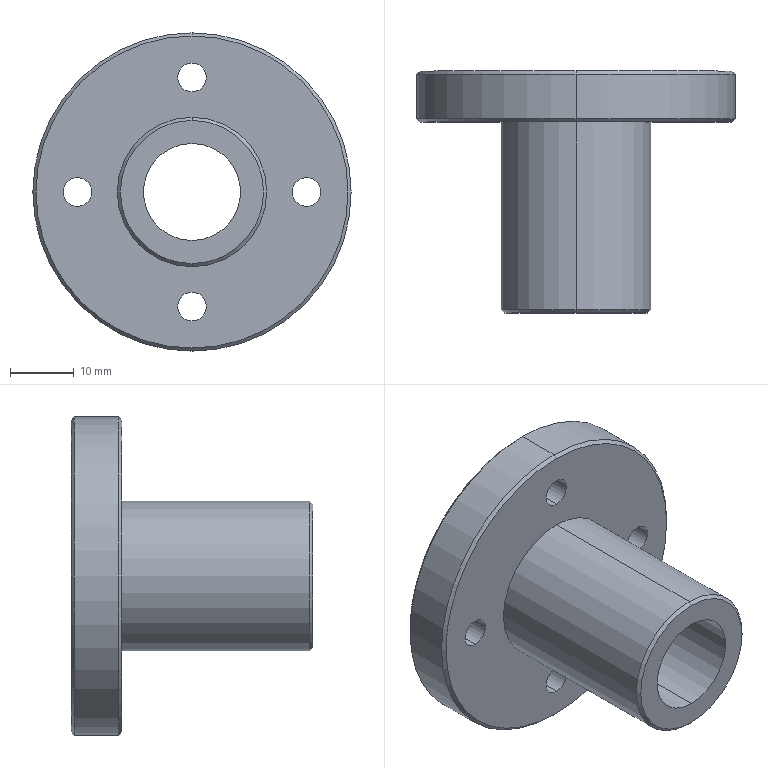Part | SolidWorks | features 3DProfileFeature 3, HoleWzd 3, Chamfer 1, Revolution 1 | 1 solid | 35 faces | box 50 x 38 x 50 mm | volume 20590 mm3 | cylinder 22 | plane 7 | cone 6 | commonest cylinder face diameters 4.5 x8 8 x8 15.25 x2 23.5 x2 50 x2
STEP:
#1=CARTESIAN_POINT('',(0.,38.,24.5));
#2=VERTEX_POINT('',#1);
#3=CARTESIAN_POINT('',(0.,38.,-24.5));
#4=VERTEX_POINT('',#3);
#5=CARTESIAN_POINT('',(0.,38.,0.));
#6=DIRECTION('',(0.,1.,0.));
#7=DIRECTION('',(0.,0.,-1.));
#8=AXIS2_PLACEMENT_3D('',#5,#6,#7);
#9=CIRCLE('',#8,24.5);
#10=EDGE_CURVE('',#2,#4,#9,.T.);
#11=ORIENTED_EDGE('',*,*,#10,.F.);
#12=CARTESIAN_POINT('',(0.,37.5,25.));
#13=VERTEX_POINT('',#12);
#14=CARTESIAN_POINT('',(0.,37.5,25.));
#15=DIRECTION('',(0.,-0.7071,0.7071));
#16=VECTOR('',#15,1000.);
#17=LINE('',#14,#16);
#18=EDGE_CURVE('',#2,#13,#17,.T.);
#19=ORIENTED_EDGE('',*,*,#18,.T.);
#20=CARTESIAN_POINT('',(0.,37.5,-25.));
#21=VERTEX_POINT('',#20);
#22=CARTESIAN_POINT('',(0.,37.5,0.));
#23=DIRECTION('',(0.,-1.,0.));
#24=DIRECTION('',(0.,0.,-1.));
#25=AXIS2_PLACEMENT_3D('',#22,#23,#24);
#26=CIRCLE('',#25,25.);
#27=EDGE_CURVE('',#21,#13,#26,.T.);
#28=ORIENTED_EDGE('',*,*,#27,.F.);
#29=CARTESIAN_POINT('',(0.,37.5,-25.));
#30=DIRECTION('',(0.,-0.7071,-0.7071));
#31=VECTOR('',#30,1000.);
#32=LINE('',#29,#31);
#33=EDGE_CURVE('',#4,#21,#32,.T.);
#34=ORIENTED_EDGE('',*,*,#33,.F.);
#35=EDGE_LOOP('',(#11,#19,#28,#34));
#36=FACE_OUTER_BOUND('',#35,.T.);
#37=CARTESIAN_POINT('',(0.,37.5,0.));
#38=DIRECTION('',(0.,-1.,0.));
#39=DIRECTION('',(0.,0.,-1.));
#40=AXIS2_PLACEMENT_3D('',#37,#38,#39);
#41=CONICAL_SURFACE('',#40,25.,0.7854);
#42=ADVANCED_FACE('',(#36),#41,.T.);
#43=CARTESIAN_POINT('',(0.,30.,-24.5));
#44=VERTEX_POINT('',#43);
#45=CARTESIAN_POINT('',(0.,30.,24.5));
#46=VERTEX_POINT('',#45);
#47=CARTESIAN_POINT('',(0.,30.,0.));
#48=DIRECTION('',(0.,-1.,0.));
#49=DIRECTION('',(0.,0.,1.));
#50=AXIS2_PLACEMENT_3D('',#47,#48,#49);
#51=CIRCLE('',#50,24.5);
#52=EDGE_CURVE('',#44,#46,#51,.T.);
#53=ORIENTED_EDGE('',*,*,#52,.F.);
#54=CARTESIAN_POINT('',(0.,30.5,-25.));
#55=VERTEX_POINT('',#54);
#56=CARTESIAN_POINT('',(0.,30.,-24.5));
#57=DIRECTION('',(0.,0.7071,-0.7071));
#58=VECTOR('',#57,1000.);
#59=LINE('',#56,#58);
#60=EDGE_CURVE('',#44,#55,#59,.T.);
#61=ORIENTED_EDGE('',*,*,#60,.T.);
#62=CARTESIAN_POINT('',(0.,30.5,25.));
#63=VERTEX_POINT('',#62);
#64=CARTESIAN_POINT('',(0.,30.5,0.));
#65=DIRECTION('',(0.,1.,0.));
#66=DIRECTION('',(0.,0.,1.));
#67=AXIS2_PLACEMENT_3D('',#64,#65,#66);
#68=CIRCLE('',#67,25.);
#69=EDGE_CURVE('',#63,#55,#68,.T.);
#70=ORIENTED_EDGE('',*,*,#69,.F.);
#71=CARTESIAN_POINT('',(0.,30.,24.5));
#72=DIRECTION('',(0.,0.7071,0.7071));
#73=VECTOR('',#72,1000.);
#74=LINE('',#71,#73);
#75=EDGE_CURVE('',#46,#63,#74,.T.);
#76=ORIENTED_EDGE('',*,*,#75,.F.);
#77=EDGE_LOOP('',(#53,#61,#70,#76));
#78=FACE_OUTER_BOUND('',#77,.T.);
#79=CARTESIAN_POINT('',(0.,30.,0.));
#80=DIRECTION('',(0.,1.,0.));
#81=DIRECTION('',(0.,0.,1.));
#82=AXIS2_PLACEMENT_3D('',#79,#80,#81);
#83=CONICAL_SURFACE('',#82,24.5,0.7854);
#84=ADVANCED_FACE('',(#78),#83,.T.);
#85=CARTESIAN_POINT('',(0.,0.,-11.25));
#86=VERTEX_POINT('',#85);
#87=CARTESIAN_POINT('',(0.,0.,11.25));
#88=VERTEX_POINT('',#87);
#89=CARTESIAN_POINT('',(0.,0.,0.));
#90=DIRECTION('',(0.,-1.,0.));
#91=DIRECTION('',(0.,0.,1.));
#92=AXIS2_PLACEMENT_3D('',#89,#90,#91);
#93=CIRCLE('',#92,11.25);
#94=EDGE_CURVE('',#86,#88,#93,.T.);
#95=ORIENTED_EDGE('',*,*,#94,.F.);
#96=CARTESIAN_POINT('',(0.,0.5,-11.75));
#97=VERTEX_POINT('',#96);
#98=CARTESIAN_POINT('',(0.,0.,-11.25));
#99=DIRECTION('',(0.,0.7071,-0.7071));
#100=VECTOR('',#99,1000.);
#101=LINE('',#98,#100);
#102=EDGE_CURVE('',#86,#97,#101,.T.);
#103=ORIENTED_EDGE('',*,*,#102,.T.);
#104=CARTESIAN_POINT('',(0.,0.5,11.75));
#105=VERTEX_POINT('',#104);
#106=CARTESIAN_POINT('',(0.,0.5,0.));
#107=DIRECTION('',(0.,1.,0.));
#108=DIRECTION('',(0.,0.,1.));
#109=AXIS2_PLACEMENT_3D('',#106,#107,#108);
#110=CIRCLE('',#109,11.75);
#111=EDGE_CURVE('',#105,#97,#110,.T.);
#112=ORIENTED_EDGE('',*,*,#111,.F.);
#113=CARTESIAN_POINT('',(0.,0.,11.25));
#114=DIRECTION('',(0.,0.7071,0.7071));
#115=VECTOR('',#114,1000.);
#116=LINE('',#113,#115);
#117=EDGE_CURVE('',#88,#105,#116,.T.);
#118=ORIENTED_EDGE('',*,*,#117,.F.);
#119=EDGE_LOOP('',(#95,#103,#112,#118));
#120=FACE_OUTER_BOUND('',#119,.T.);
#121=CARTESIAN_POINT('',(0.,0.,0.));
#122=DIRECTION('',(0.,1.,0.));
#123=DIRECTION('',(0.,0.,1.));
#124=AXIS2_PLACEMENT_3D('',#121,#122,#123);
#125=CONICAL_SURFACE('',#124,11.25,0.7854);
#126=ADVANCED_FACE('',(#120),#125,.T.);
#127=CARTESIAN_POINT('',(0.,33.4,-22.));
#128=VERTEX_POINT('',#127);
#129=CARTESIAN_POINT('',(0.,33.4,-14.));
#130=VERTEX_POINT('',#129);
#131=CARTESIAN_POINT('',(0.,33.4,-18.));
#132=DIRECTION('',(0.,1.,0.));
#133=DIRECTION('',(0.,0.,1.));
#134=AXIS2_PLACEMENT_3D('',#131,#132,#133);
#135=CIRCLE('',#134,4.);
#136=EDGE_CURVE('',#128,#130,#135,.T.);
#137=ORIENTED_EDGE('',*,*,#136,.F.);
#138=CARTESIAN_POINT('',(0.,38.,-22.));
#139=VERTEX_POINT('',#138);
#140=CARTESIAN_POINT('',(0.,38.,-22.));
#141=DIRECTION('',(0.,1.,0.));
#142=VECTOR('',#141,1000.);
#143=LINE('',#140,#142);
#144=EDGE_CURVE('',#128,#139,#143,.T.);
#145=ORIENTED_EDGE('',*,*,#144,.T.);
#146=CARTESIAN_POINT('',(0.,38.,-14.));
#147=VERTEX_POINT('',#146);
#148=CARTESIAN_POINT('',(0.,38.,-18.));
#149=DIRECTION('',(0.,1.,0.));
#150=DIRECTION('',(0.,0.,1.));
#151=AXIS2_PLACEMENT_3D('',#148,#149,#150);
#152=CIRCLE('',#151,4.);
#153=EDGE_CURVE('',#139,#147,#152,.T.);
#154=ORIENTED_EDGE('',*,*,#153,.T.);
#155=CARTESIAN_POINT('',(0.,38.,-14.));
#156=DIRECTION('',(0.,1.,0.));
#157=VECTOR('',#156,1000.);
#158=LINE('',#155,#157);
#159=EDGE_CURVE('',#130,#147,#158,.T.);
#160=ORIENTED_EDGE('',*,*,#159,.F.);
#161=EDGE_LOOP('',(#137,#145,#154,#160));
#162=FACE_OUTER_BOUND('',#161,.T.);
#163=CARTESIAN_POINT('',(0.,38.,-18.));
#164=DIRECTION('',(0.,1.,0.));
#165=DIRECTION('',(0.,0.,1.));
#166=AXIS2_PLACEMENT_3D('',#163,#164,#165);
#167=CYLINDRICAL_SURFACE('',#166,4.);
#168=ADVANCED_FACE('',(#162),#167,.F.);
#169=CARTESIAN_POINT('',(0.,30.,-20.25));
#170=VERTEX_POINT('',#169);
#171=CARTESIAN_POINT('',(0.,30.,-15.75));
#172=VERTEX_POINT('',#171);
#173=CARTESIAN_POINT('',(0.,30.,-18.));
#174=DIRECTION('',(0.,1.,0.));
#175=DIRECTION('',(0.,0.,1.));
#176=AXIS2_PLACEMENT_3D('',#173,#174,#175);
#177=CIRCLE('',#176,2.25);
#178=EDGE_CURVE('',#170,#172,#177,.T.);
#179=ORIENTED_EDGE('',*,*,#178,.F.);
#180=CARTESIAN_POINT('',(0.,33.4,-20.25));
#181=VERTEX_POINT('',#180);
#182=CARTESIAN_POINT('',(0.,38.,-20.25));
#183=DIRECTION('',(0.,1.,0.));
#184=VECTOR('',#183,1000.);
#185=LINE('',#182,#184);
#186=EDGE_CURVE('',#170,#181,#185,.T.);
#187=ORIENTED_EDGE('',*,*,#186,.T.);
#188=CARTESIAN_POINT('',(0.,33.4,-15.75));
#189=VERTEX_POINT('',#188);
#190=CARTESIAN_POINT('',(0.,33.4,-18.));
#191=DIRECTION('',(0.,1.,0.));
#192=DIRECTION('',(0.,0.,1.));
#193=AXIS2_PLACEMENT_3D('',#190,#191,#192);
#194=CIRCLE('',#193,2.25);
#195=EDGE_CURVE('',#181,#189,#194,.T.);
#196=ORIENTED_EDGE('',*,*,#195,.T.);
#197=CARTESIAN_POINT('',(0.,38.,-15.75));
#198=DIRECTION('',(0.,1.,0.));
#199=VECTOR('',#198,1000.);
#200=LINE('',#197,#199);
#201=EDGE_CURVE('',#172,#189,#200,.T.);
#202=ORIENTED_EDGE('',*,*,#201,.F.);
#203=EDGE_LOOP('',(#179,#187,#196,#202));
#204=FACE_OUTER_BOUND('',#203,.T.);
#205=CARTESIAN_POINT('',(0.,38.,-18.));
#206=DIRECTION('',(0.,1.,0.));
#207=DIRECTION('',(0.,0.,1.));
#208=AXIS2_PLACEMENT_3D('',#205,#206,#207);
#209=CYLINDRICAL_SURFACE('',#208,2.25);
#210=ADVANCED_FACE('',(#204),#209,.F.);
#211=CARTESIAN_POINT('',(-18.,33.4,-4.));
#212=VERTEX_POINT('',#211);
#213=CARTESIAN_POINT('',(-18.,33.4,4.));
#214=VERTEX_POINT('',#213);
#215=CARTESIAN_POINT('',(-18.,33.4,0.));
#216=DIRECTION('',(0.,1.,0.));
#217=DIRECTION('',(0.,0.,1.));
#218=AXIS2_PLACEMENT_3D('',#215,#216,#217);
#219=CIRCLE('',#218,4.);
#220=EDGE_CURVE('',#212,#214,#219,.T.);
#221=ORIENTED_EDGE('',*,*,#220,.F.);
#222=CARTESIAN_POINT('',(-18.,38.,-4.));
#223=VERTEX_POINT('',#222);
#224=CARTESIAN_POINT('',(-18.,38.,-4.));
#225=DIRECTION('',(0.,1.,0.));
#226=VECTOR('',#225,1000.);
#227=LINE('',#224,#226);
#228=EDGE_CURVE('',#212,#223,#227,.T.);
#229=ORIENTED_EDGE('',*,*,#228,.T.);
#230=CARTESIAN_POINT('',(-18.,38.,4.));
#231=VERTEX_POINT('',#230);
#232=CARTESIAN_POINT('',(-18.,38.,0.));
#233=DIRECTION('',(0.,1.,0.));
#234=DIRECTION('',(0.,0.,1.));
#235=AXIS2_PLACEMENT_3D('',#232,#233,#234);
#236=CIRCLE('',#235,4.);
#237=EDGE_CURVE('',#223,#231,#236,.T.);
#238=ORIENTED_EDGE('',*,*,#237,.T.);
#239=CARTESIAN_POINT('',(-18.,38.,4.));
#240=DIRECTION('',(0.,1.,0.));
#241=VECTOR('',#240,1000.);
#242=LINE('',#239,#241);
#243=EDGE_CURVE('',#214,#231,#242,.T.);
#244=ORIENTED_EDGE('',*,*,#243,.F.);
#245=EDGE_LOOP('',(#221,#229,#238,#244));
#246=FACE_OUTER_BOUND('',#245,.T.);
#247=CARTESIAN_POINT('',(-18.,38.,0.));
#248=DIRECTION('',(0.,1.,0.));
#249=DIRECTION('',(0.,0.,1.));
#250=AXIS2_PLACEMENT_3D('',#247,#248,#249);
#251=CYLINDRICAL_SURFACE('',#250,4.);
#252=ADVANCED_FACE('',(#246),#251,.F.);
#253=CARTESIAN_POINT('',(-18.,30.,-2.25));
#254=VERTEX_POINT('',#253);
#255=CARTESIAN_POINT('',(-18.,30.,2.25));
#256=VERTEX_POINT('',#255);
#257=CARTESIAN_POINT('',(-18.,30.,0.));
#258=DIRECTION('',(0.,1.,0.));
#259=DIRECTION('',(0.,0.,1.));
#260=AXIS2_PLACEMENT_3D('',#257,#258,#259);
#261=CIRCLE('',#260,2.25);
#262=EDGE_CURVE('',#254,#256,#261,.T.);
#263=ORIENTED_EDGE('',*,*,#262,.F.);
#264=CARTESIAN_POINT('',(-18.,33.4,-2.25));
#265=VERTEX_POINT('',#264);
#266=CARTESIAN_POINT('',(-18.,38.,-2.25));
#267=DIRECTION('',(0.,1.,0.));
#268=VECTOR('',#267,1000.);
#269=LINE('',#266,#268);
#270=EDGE_CURVE('',#254,#265,#269,.T.);
#271=ORIENTED_EDGE('',*,*,#270,.T.);
#272=CARTESIAN_POINT('',(-18.,33.4,2.25));
#273=VERTEX_POINT('',#272);
#274=CARTESIAN_POINT('',(-18.,33.4,0.));
#275=DIRECTION('',(0.,1.,0.));
#276=DIRECTION('',(0.,0.,1.));
#277=AXIS2_PLACEMENT_3D('',#274,#275,#276);
#278=CIRCLE('',#277,2.25);
#279=EDGE_CURVE('',#265,#273,#278,.T.);
#280=ORIENTED_EDGE('',*,*,#279,.T.);
#281=CARTESIAN_POINT('',(-18.,38.,2.25));
#282=DIRECTION('',(0.,1.,0.));
#283=VECTOR('',#282,1000.);
#284=LINE('',#281,#283);
#285=EDGE_CURVE('',#256,#273,#284,.T.);
#286=ORIENTED_EDGE('',*,*,#285,.F.);
#287=EDGE_LOOP('',(#263,#271,#280,#286));
#288=FACE_OUTER_BOUND('',#287,.T.);
#289=CARTESIAN_POINT('',(-18.,38.,0.));
#290=DIRECTION('',(0.,1.,0.));
#291=DIRECTION('',(0.,0.,1.));
#292=AXIS2_PLACEMENT_3D('',#289,#290,#291);
#293=CYLINDRICAL_SURFACE('',#292,2.25);
#294=ADVANCED_FACE('',(#288),#293,.F.);
#295=CARTESIAN_POINT('',(18.,33.4,-4.));
#296=VERTEX_POINT('',#295);
#297=CARTESIAN_POINT('',(18.,33.4,4.));
#298=VERTEX_POINT('',#297);
#299=CARTESIAN_POINT('',(18.,33.4,0.));
#300=DIRECTION('',(0.,1.,0.));
#301=DIRECTION('',(0.,0.,1.));
#302=AXIS2_PLACEMENT_3D('',#299,#300,#301);
#303=CIRCLE('',#302,4.);
#304=EDGE_CURVE('',#296,#298,#303,.T.);
#305=ORIENTED_EDGE('',*,*,#304,.F.);
#306=CARTESIAN_POINT('',(18.,38.,-4.));
#307=VERTEX_POINT('',#306);
#308=CARTESIAN_POINT('',(18.,38.,-4.));
#309=DIRECTION('',(0.,1.,0.));
#310=VECTOR('',#309,1000.);
#311=LINE('',#308,#310);
#312=EDGE_CURVE('',#296,#307,#311,.T.);
#313=ORIENTED_EDGE('',*,*,#312,.T.);
#314=CARTESIAN_POINT('',(18.,38.,4.));
#315=VERTEX_POINT('',#314);
#316=CARTESIAN_POINT('',(18.,38.,0.));
#317=DIRECTION('',(0.,1.,0.));
#318=DIRECTION('',(0.,0.,1.));
#319=AXIS2_PLACEMENT_3D('',#316,#317,#318);
#320=CIRCLE('',#319,4.);
#321=EDGE_CURVE('',#307,#315,#320,.T.);
#322=ORIENTED_EDGE('',*,*,#321,.T.);
#323=CARTESIAN_POINT('',(18.,38.,4.));
#324=DIRECTION('',(0.,1.,0.));
#325=VECTOR('',#324,1000.);
#326=LINE('',#323,#325);
#327=EDGE_CURVE('',#298,#315,#326,.T.);
#328=ORIENTED_EDGE('',*,*,#327,.F.);
#329=EDGE_LOOP('',(#305,#313,#322,#328));
#330=FACE_OUTER_BOUND('',#329,.T.);
#331=CARTESIAN_POINT('',(18.,38.,0.));
#332=DIRECTION('',(0.,1.,0.));
#333=DIRECTION('',(0.,0.,1.));
#334=AXIS2_PLACEMENT_3D('',#331,#332,#333);
#335=CYLINDRICAL_SURFACE('',#334,4.);
#336=ADVANCED_FACE('',(#330),#335,.F.);
#337=CARTESIAN_POINT('',(18.,30.,-2.25));
#338=VERTEX_POINT('',#337);
#339=CARTESIAN_POINT('',(18.,30.,2.25));
#340=VERTEX_POINT('',#339);
#341=CARTESIAN_POINT('',(18.,30.,0.));
#342=DIRECTION('',(0.,1.,0.));
#343=DIRECTION('',(0.,0.,1.));
#344=AXIS2_PLACEMENT_3D('',#341,#342,#343);
#345=CIRCLE('',#344,2.25);
#346=EDGE_CURVE('',#338,#340,#345,.T.);
#347=ORIENTED_EDGE('',*,*,#346,.F.);
#348=CARTESIAN_POINT('',(18.,33.4,-2.25));
#349=VERTEX_POINT('',#348);
#350=CARTESIAN_POINT('',(18.,38.,-2.25));
#351=DIRECTION('',(0.,1.,0.));
#352=VECTOR('',#351,1000.);
#353=LINE('',#350,#352);
#354=EDGE_CURVE('',#338,#349,#353,.T.);
#355=ORIENTED_EDGE('',*,*,#354,.T.);
#356=CARTESIAN_POINT('',(18.,33.4,2.25));
#357=VERTEX_POINT('',#356);
#358=CARTESIAN_POINT('',(18.,33.4,0.));
#359=DIRECTION('',(0.,1.,0.));
#360=DIRECTION('',(0.,0.,1.));
#361=AXIS2_PLACEMENT_3D('',#358,#359,#360);
#362=CIRCLE('',#361,2.25);
#363=EDGE_CURVE('',#349,#357,#362,.T.);
#364=ORIENTED_EDGE('',*,*,#363,.T.);
#365=CARTESIAN_POINT('',(18.,38.,2.25));
#366=DIRECTION('',(0.,1.,0.));
#367=VECTOR('',#366,1000.);
#368=LINE('',#365,#367);
#369=EDGE_CURVE('',#340,#357,#368,.T.);
#370=ORIENTED_EDGE('',*,*,#369,.F.);
#371=EDGE_LOOP('',(#347,#355,#364,#370));
#372=FACE_OUTER_BOUND('',#371,.T.);
#373=CARTESIAN_POINT('',(18.,38.,0.));
#374=DIRECTION('',(0.,1.,0.));
#375=DIRECTION('',(0.,0.,1.));
#376=AXIS2_PLACEMENT_3D('',#373,#374,#375);
#377=CYLINDRICAL_SURFACE('',#376,2.25);
#378=ADVANCED_FACE('',(#372),#377,.F.);
#379=CARTESIAN_POINT('',(0.,33.4,14.));
#380=VERTEX_POINT('',#379);
#381=CARTESIAN_POINT('',(0.,33.4,22.));
#382=VERTEX_POINT('',#381);
#383=CARTESIAN_POINT('',(0.,33.4,18.));
#384=DIRECTION('',(0.,1.,0.));
#385=DIRECTION('',(0.,0.,1.));
#386=AXIS2_PLACEMENT_3D('',#383,#384,#385);
#387=CIRCLE('',#386,4.);
#388=EDGE_CURVE('',#380,#382,#387,.T.);
#389=ORIENTED_EDGE('',*,*,#388,.F.);
#390=CARTESIAN_POINT('',(0.,38.,14.));
#391=VERTEX_POINT('',#390);
#392=CARTESIAN_POINT('',(0.,38.,14.));
#393=DIRECTION('',(0.,1.,0.));
#394=VECTOR('',#393,1000.);
#395=LINE('',#392,#394);
#396=EDGE_CURVE('',#380,#391,#395,.T.);
#397=ORIENTED_EDGE('',*,*,#396,.T.);
#398=CARTESIAN_POINT('',(0.,38.,22.));
#399=VERTEX_POINT('',#398);
#400=CARTESIAN_POINT('',(0.,38.,18.));
#401=DIRECTION('',(0.,1.,0.));
#402=DIRECTION('',(0.,0.,1.));
#403=AXIS2_PLACEMENT_3D('',#400,#401,#402);
#404=CIRCLE('',#403,4.);
#405=EDGE_CURVE('',#391,#399,#404,.T.);
#406=ORIENTED_EDGE('',*,*,#405,.T.);
#407=CARTESIAN_POINT('',(0.,38.,22.));
#408=DIRECTION('',(0.,1.,0.));
#409=VECTOR('',#408,1000.);
#410=LINE('',#407,#409);
#411=EDGE_CURVE('',#382,#399,#410,.T.);
#412=ORIENTED_EDGE('',*,*,#411,.F.);
#413=EDGE_LOOP('',(#389,#397,#406,#412));
#414=FACE_OUTER_BOUND('',#413,.T.);
#415=CARTESIAN_POINT('',(0.,38.,18.));
#416=DIRECTION('',(0.,1.,0.));
#417=DIRECTION('',(0.,0.,1.));
#418=AXIS2_PLACEMENT_3D('',#415,#416,#417);
#419=CYLINDRICAL_SURFACE('',#418,4.);
#420=ADVANCED_FACE('',(#414),#419,.F.);
#421=CARTESIAN_POINT('',(0.,30.,15.75));
#422=VERTEX_POINT('',#421);
#423=CARTESIAN_POINT('',(0.,30.,20.25));
#424=VERTEX_POINT('',#423);
#425=CARTESIAN_POINT('',(0.,30.,18.));
#426=DIRECTION('',(0.,1.,0.));
#427=DIRECTION('',(0.,0.,1.));
#428=AXIS2_PLACEMENT_3D('',#425,#426,#427);
#429=CIRCLE('',#428,2.25);
#430=EDGE_CURVE('',#422,#424,#429,.T.);
#431=ORIENTED_EDGE('',*,*,#430,.F.);
#432=CARTESIAN_POINT('',(0.,33.4,15.75));
#433=VERTEX_POINT('',#432);
#434=CARTESIAN_POINT('',(0.,38.,15.75));
#435=DIRECTION('',(0.,1.,0.));
#436=VECTOR('',#435,1000.);
#437=LINE('',#434,#436);
#438=EDGE_CURVE('',#422,#433,#437,.T.);
#439=ORIENTED_EDGE('',*,*,#438,.T.);
#440=CARTESIAN_POINT('',(0.,33.4,20.25));
#441=VERTEX_POINT('',#440);
#442=CARTESIAN_POINT('',(0.,33.4,18.));
#443=DIRECTION('',(0.,1.,0.));
#444=DIRECTION('',(0.,0.,1.));
#445=AXIS2_PLACEMENT_3D('',#442,#443,#444);
#446=CIRCLE('',#445,2.25);
#447=EDGE_CURVE('',#433,#441,#446,.T.);
#448=ORIENTED_EDGE('',*,*,#447,.T.);
#449=CARTESIAN_POINT('',(0.,38.,20.25));
#450=DIRECTION('',(0.,1.,0.));
#451=VECTOR('',#450,1000.);
#452=LINE('',#449,#451);
#453=EDGE_CURVE('',#424,#441,#452,.T.);
#454=ORIENTED_EDGE('',*,*,#453,.F.);
#455=EDGE_LOOP('',(#431,#439,#448,#454));
#456=FACE_OUTER_BOUND('',#455,.T.);
#457=CARTESIAN_POINT('',(0.,38.,18.));
#458=DIRECTION('',(0.,1.,0.));
#459=DIRECTION('',(0.,0.,1.));
#460=AXIS2_PLACEMENT_3D('',#457,#458,#459);
#461=CYLINDRICAL_SURFACE('',#460,2.25);
#462=ADVANCED_FACE('',(#456),#461,.F.);
#463=CARTESIAN_POINT('',(0.,0.,-7.625));
#464=VERTEX_POINT('',#463);
#465=CARTESIAN_POINT('',(0.,0.,7.625));
#466=VERTEX_POINT('',#465);
#467=CARTESIAN_POINT('',(0.,0.,0.));
#468=DIRECTION('',(0.,1.,0.));
#469=DIRECTION('',(0.,0.,1.));
#470=AXIS2_PLACEMENT_3D('',#467,#468,#469);
#471=CIRCLE('',#470,7.625);
#472=EDGE_CURVE('',#464,#466,#471,.T.);
#473=ORIENTED_EDGE('',*,*,#472,.F.);
#474=CARTESIAN_POINT('',(0.,38.,-7.625));
#475=VERTEX_POINT('',#474);
#476=CARTESIAN_POINT('',(0.,38.,-7.625));
#477=DIRECTION('',(0.,1.,0.));
#478=VECTOR('',#477,1000.);
#479=LINE('',#476,#478);
#480=EDGE_CURVE('',#464,#475,#479,.T.);
#481=ORIENTED_EDGE('',*,*,#480,.T.);
#482=CARTESIAN_POINT('',(0.,38.,7.625));
#483=VERTEX_POINT('',#482);
#484=CARTESIAN_POINT('',(0.,38.,0.));
#485=DIRECTION('',(0.,1.,0.));
#486=DIRECTION('',(0.,0.,1.));
#487=AXIS2_PLACEMENT_3D('',#484,#485,#486);
#488=CIRCLE('',#487,7.625);
#489=EDGE_CURVE('',#475,#483,#488,.T.);
#490=ORIENTED_EDGE('',*,*,#489,.T.);
#491=CARTESIAN_POINT('',(0.,38.,7.625));
#492=DIRECTION('',(0.,1.,0.));
#493=VECTOR('',#492,1000.);
#494=LINE('',#491,#493);
#495=EDGE_CURVE('',#466,#483,#494,.T.);
#496=ORIENTED_EDGE('',*,*,#495,.F.);
#497=EDGE_LOOP('',(#473,#481,#490,#496));
#498=FACE_OUTER_BOUND('',#497,.T.);
#499=CARTESIAN_POINT('',(0.,38.,0.));
#500=DIRECTION('',(0.,1.,0.));
#501=DIRECTION('',(0.,0.,1.));
#502=AXIS2_PLACEMENT_3D('',#499,#500,#501);
#503=CYLINDRICAL_SURFACE('',#502,7.625);
#504=ADVANCED_FACE('',(#498),#503,.F.);
#505=CARTESIAN_POINT('',(0.,30.,-11.75));
#506=VERTEX_POINT('',#505);
#507=CARTESIAN_POINT('',(0.,30.,11.75));
#508=VERTEX_POINT('',#507);
#509=CARTESIAN_POINT('',(0.,30.,0.));
#510=DIRECTION('',(0.,-1.,0.));
#511=DIRECTION('',(0.,0.,-1.));
#512=AXIS2_PLACEMENT_3D('',#509,#510,#511);
#513=CIRCLE('',#512,11.75);
#514=EDGE_CURVE('',#506,#508,#513,.T.);
#515=ORIENTED_EDGE('',*,*,#514,.T.);
#516=CARTESIAN_POINT('',(0.,0.,11.75));
#517=DIRECTION('',(0.,-1.,0.));
#518=VECTOR('',#517,1000.);
#519=LINE('',#516,#518);
#520=EDGE_CURVE('',#508,#105,#519,.T.);
#521=ORIENTED_EDGE('',*,*,#520,.T.);
#522=ORIENTED_EDGE('',*,*,#111,.T.);
#523=CARTESIAN_POINT('',(0.,0.,-11.75));
#524=DIRECTION('',(0.,-1.,0.));
#525=VECTOR('',#524,1000.);
#526=LINE('',#523,#525);
#527=EDGE_CURVE('',#506,#97,#526,.T.);
#528=ORIENTED_EDGE('',*,*,#527,.F.);
#529=EDGE_LOOP('',(#515,#521,#522,#528));
#530=FACE_OUTER_BOUND('',#529,.T.);
#531=CARTESIAN_POINT('',(0.,0.,0.));
#532=DIRECTION('',(0.,-1.,0.));
#533=DIRECTION('',(0.,0.,-1.));
#534=AXIS2_PLACEMENT_3D('',#531,#532,#533);
#535=CYLINDRICAL_SURFACE('',#534,11.75);
#536=ADVANCED_FACE('',(#530),#535,.T.);
#537=ORIENTED_EDGE('',*,*,#27,.T.);
#538=CARTESIAN_POINT('',(0.,0.,25.));
#539=DIRECTION('',(0.,-1.,0.));
#540=VECTOR('',#539,1000.);
#541=LINE('',#538,#540);
#542=EDGE_CURVE('',#13,#63,#541,.T.);
#543=ORIENTED_EDGE('',*,*,#542,.T.);
#544=ORIENTED_EDGE('',*,*,#69,.T.);
#545=CARTESIAN_POINT('',(0.,0.,-25.));
#546=DIRECTION('',(0.,-1.,0.));
#547=VECTOR('',#546,1000.);
#548=LINE('',#545,#547);
#549=EDGE_CURVE('',#21,#55,#548,.T.);
#550=ORIENTED_EDGE('',*,*,#549,.F.);
#551=EDGE_LOOP('',(#537,#543,#544,#550));
#552=FACE_OUTER_BOUND('',#551,.T.);
#553=CARTESIAN_POINT('',(0.,0.,0.));
#554=DIRECTION('',(0.,-1.,0.));
#555=DIRECTION('',(0.,0.,-1.));
#556=AXIS2_PLACEMENT_3D('',#553,#554,#555);
#557=CYLINDRICAL_SURFACE('',#556,25.);
#558=ADVANCED_FACE('',(#552),#557,.T.);
#559=CARTESIAN_POINT('',(0.,38.,0.));
#560=DIRECTION('',(0.,1.,0.));
#561=DIRECTION('',(0.,0.,-1.));
#562=AXIS2_PLACEMENT_3D('',#559,#560,#561);
#563=CIRCLE('',#562,24.5);
#564=EDGE_CURVE('',#4,#2,#563,.T.);
#565=ORIENTED_EDGE('',*,*,#564,.T.);
#566=ORIENTED_EDGE('',*,*,#10,.T.);
#567=EDGE_LOOP('',(#565,#566));
#568=FACE_OUTER_BOUND('',#567,.T.);
#569=CARTESIAN_POINT('',(0.,38.,-18.));
#570=DIRECTION('',(0.,1.,0.));
#571=DIRECTION('',(0.,0.,1.));
#572=AXIS2_PLACEMENT_3D('',#569,#570,#571);
#573=CIRCLE('',#572,4.);
#574=EDGE_CURVE('',#147,#139,#573,.T.);
#575=ORIENTED_EDGE('',*,*,#574,.F.);
#576=ORIENTED_EDGE('',*,*,#153,.F.);
#577=EDGE_LOOP('',(#575,#576));
#578=FACE_BOUND('',#577,.T.);
#579=CARTESIAN_POINT('',(-18.,38.,0.));
#580=DIRECTION('',(0.,1.,0.));
#581=DIRECTION('',(0.,0.,1.));
#582=AXIS2_PLACEMENT_3D('',#579,#580,#581);
#583=CIRCLE('',#582,4.);
#584=EDGE_CURVE('',#231,#223,#583,.T.);
#585=ORIENTED_EDGE('',*,*,#584,.F.);
#586=ORIENTED_EDGE('',*,*,#237,.F.);
#587=EDGE_LOOP('',(#585,#586));
#588=FACE_BOUND('',#587,.T.);
#589=CARTESIAN_POINT('',(18.,38.,0.));
#590=DIRECTION('',(0.,1.,0.));
#591=DIRECTION('',(0.,0.,1.));
#592=AXIS2_PLACEMENT_3D('',#589,#590,#591);
#593=CIRCLE('',#592,4.);
#594=EDGE_CURVE('',#315,#307,#593,.T.);
#595=ORIENTED_EDGE('',*,*,#594,.F.);
#596=ORIENTED_EDGE('',*,*,#321,.F.);
#597=EDGE_LOOP('',(#595,#596));
#598=FACE_BOUND('',#597,.T.);
#599=CARTESIAN_POINT('',(0.,38.,18.));
#600=DIRECTION('',(0.,1.,0.));
#601=DIRECTION('',(0.,0.,1.));
#602=AXIS2_PLACEMENT_3D('',#599,#600,#601);
#603=CIRCLE('',#602,4.);
#604=EDGE_CURVE('',#399,#391,#603,.T.);
#605=ORIENTED_EDGE('',*,*,#604,.F.);
#606=ORIENTED_EDGE('',*,*,#405,.F.);
#607=EDGE_LOOP('',(#605,#606));
#608=FACE_BOUND('',#607,.T.);
#609=CARTESIAN_POINT('',(0.,38.,0.));
#610=DIRECTION('',(0.,1.,0.));
#611=DIRECTION('',(0.,0.,1.));
#612=AXIS2_PLACEMENT_3D('',#609,#610,#611);
#613=CIRCLE('',#612,7.625);
#614=EDGE_CURVE('',#483,#475,#613,.T.);
#615=ORIENTED_EDGE('',*,*,#614,.F.);
#616=ORIENTED_EDGE('',*,*,#489,.F.);
#617=EDGE_LOOP('',(#615,#616));
#618=FACE_BOUND('',#617,.T.);
#619=CARTESIAN_POINT('',(0.,38.,0.));
#620=DIRECTION('',(0.,-1.,0.));
#621=DIRECTION('',(0.,0.,-1.));
#622=AXIS2_PLACEMENT_3D('',#619,#620,#621);
#623=PLANE('',#622);
#624=ADVANCED_FACE('',(#568,#578,#588,#598,#608,#618),#623,.F.);
#625=ORIENTED_EDGE('',*,*,#542,.F.);
#626=CARTESIAN_POINT('',(0.,37.5,0.));
#627=DIRECTION('',(0.,-1.,0.));
#628=DIRECTION('',(0.,0.,-1.));
#629=AXIS2_PLACEMENT_3D('',#626,#627,#628);
#630=CIRCLE('',#629,25.);
#631=EDGE_CURVE('',#13,#21,#630,.T.);
#632=ORIENTED_EDGE('',*,*,#631,.T.);
#633=ORIENTED_EDGE('',*,*,#549,.T.);
#634=CARTESIAN_POINT('',(0.,30.5,0.));
#635=DIRECTION('',(0.,1.,0.));
#636=DIRECTION('',(0.,0.,1.));
#637=AXIS2_PLACEMENT_3D('',#634,#635,#636);
#638=CIRCLE('',#637,25.);
#639=EDGE_CURVE('',#55,#63,#638,.T.);
#640=ORIENTED_EDGE('',*,*,#639,.T.);
#641=EDGE_LOOP('',(#625,#632,#633,#640));
#642=FACE_OUTER_BOUND('',#641,.T.);
#643=CARTESIAN_POINT('',(0.,0.,0.));
#644=DIRECTION('',(0.,-1.,0.));
#645=DIRECTION('',(0.,0.,-1.));
#646=AXIS2_PLACEMENT_3D('',#643,#644,#645);
#647=CYLINDRICAL_SURFACE('',#646,25.);
#648=ADVANCED_FACE('',(#642),#647,.T.);
#649=CARTESIAN_POINT('',(0.,30.,0.));
#650=DIRECTION('',(0.,-1.,0.));
#651=DIRECTION('',(0.,0.,1.));
#652=AXIS2_PLACEMENT_3D('',#649,#650,#651);
#653=CIRCLE('',#652,24.5);
#654=EDGE_CURVE('',#46,#44,#653,.T.);
#655=ORIENTED_EDGE('',*,*,#654,.T.);
#656=ORIENTED_EDGE('',*,*,#52,.T.);
#657=EDGE_LOOP('',(#655,#656));
#658=FACE_OUTER_BOUND('',#657,.T.);
#659=CARTESIAN_POINT('',(0.,30.,-18.));
#660=DIRECTION('',(0.,1.,0.));
#661=DIRECTION('',(0.,0.,1.));
#662=AXIS2_PLACEMENT_3D('',#659,#660,#661);
#663=CIRCLE('',#662,2.25);
#664=EDGE_CURVE('',#172,#170,#663,.T.);
#665=ORIENTED_EDGE('',*,*,#664,.T.);
#666=ORIENTED_EDGE('',*,*,#178,.T.);
#667=EDGE_LOOP('',(#665,#666));
#668=FACE_BOUND('',#667,.T.);
#669=CARTESIAN_POINT('',(-18.,30.,0.));
#670=DIRECTION('',(0.,1.,0.));
#671=DIRECTION('',(0.,0.,1.));
#672=AXIS2_PLACEMENT_3D('',#669,#670,#671);
#673=CIRCLE('',#672,2.25);
#674=EDGE_CURVE('',#256,#254,#673,.T.);
#675=ORIENTED_EDGE('',*,*,#674,.T.);
#676=ORIENTED_EDGE('',*,*,#262,.T.);
#677=EDGE_LOOP('',(#675,#676));
#678=FACE_BOUND('',#677,.T.);
#679=CARTESIAN_POINT('',(18.,30.,0.));
#680=DIRECTION('',(0.,1.,0.));
#681=DIRECTION('',(0.,0.,1.));
#682=AXIS2_PLACEMENT_3D('',#679,#680,#681);
#683=CIRCLE('',#682,2.25);
#684=EDGE_CURVE('',#340,#338,#683,.T.);
#685=ORIENTED_EDGE('',*,*,#684,.T.);
#686=ORIENTED_EDGE('',*,*,#346,.T.);
#687=EDGE_LOOP('',(#685,#686));
#688=FACE_BOUND('',#687,.T.);
#689=CARTESIAN_POINT('',(0.,30.,18.));
#690=DIRECTION('',(0.,1.,0.));
#691=DIRECTION('',(0.,0.,1.));
#692=AXIS2_PLACEMENT_3D('',#689,#690,#691);
#693=CIRCLE('',#692,2.25);
#694=EDGE_CURVE('',#424,#422,#693,.T.);
#695=ORIENTED_EDGE('',*,*,#694,.T.);
#696=ORIENTED_EDGE('',*,*,#430,.T.);
#697=EDGE_LOOP('',(#695,#696));
#698=FACE_BOUND('',#697,.T.);
#699=ORIENTED_EDGE('',*,*,#514,.F.);
#700=CARTESIAN_POINT('',(0.,30.,0.));
#701=DIRECTION('',(0.,-1.,0.));
#702=DIRECTION('',(0.,0.,-1.));
#703=AXIS2_PLACEMENT_3D('',#700,#701,#702);
#704=CIRCLE('',#703,11.75);
#705=EDGE_CURVE('',#508,#506,#704,.T.);
#706=ORIENTED_EDGE('',*,*,#705,.F.);
#707=EDGE_LOOP('',(#699,#706));
#708=FACE_BOUND('',#707,.T.);
#709=CARTESIAN_POINT('',(-25.,30.,0.));
#710=DIRECTION('',(0.,1.,0.));
#711=DIRECTION('',(0.,0.,1.));
#712=AXIS2_PLACEMENT_3D('',#709,#710,#711);
#713=PLANE('',#712);
#714=ADVANCED_FACE('',(#658,#668,#678,#688,#698,#708),#713,.F.);
#715=ORIENTED_EDGE('',*,*,#520,.F.);
#716=ORIENTED_EDGE('',*,*,#705,.T.);
#717=ORIENTED_EDGE('',*,*,#527,.T.);
#718=CARTESIAN_POINT('',(0.,0.5,0.));
#719=DIRECTION('',(0.,1.,0.));
#720=DIRECTION('',(0.,0.,1.));
#721=AXIS2_PLACEMENT_3D('',#718,#719,#720);
#722=CIRCLE('',#721,11.75);
#723=EDGE_CURVE('',#97,#105,#722,.T.);
#724=ORIENTED_EDGE('',*,*,#723,.T.);
#725=EDGE_LOOP('',(#715,#716,#717,#724));
#726=FACE_OUTER_BOUND('',#725,.T.);
#727=CARTESIAN_POINT('',(0.,0.,0.));
#728=DIRECTION('',(0.,-1.,0.));
#729=DIRECTION('',(0.,0.,-1.));
#730=AXIS2_PLACEMENT_3D('',#727,#728,#729);
#731=CYLINDRICAL_SURFACE('',#730,11.75);
#732=ADVANCED_FACE('',(#726),#731,.T.);
#733=CARTESIAN_POINT('',(0.,0.,0.));
#734=DIRECTION('',(0.,-1.,0.));
#735=DIRECTION('',(0.,0.,1.));
#736=AXIS2_PLACEMENT_3D('',#733,#734,#735);
#737=CIRCLE('',#736,11.25);
#738=EDGE_CURVE('',#88,#86,#737,.T.);
#739=ORIENTED_EDGE('',*,*,#738,.T.);
#740=ORIENTED_EDGE('',*,*,#94,.T.);
#741=EDGE_LOOP('',(#739,#740));
#742=FACE_OUTER_BOUND('',#741,.T.);
#743=CARTESIAN_POINT('',(0.,0.,0.));
#744=DIRECTION('',(0.,1.,0.));
#745=DIRECTION('',(0.,0.,1.));
#746=AXIS2_PLACEMENT_3D('',#743,#744,#745);
#747=CIRCLE('',#746,7.625);
#748=EDGE_CURVE('',#466,#464,#747,.T.);
#749=ORIENTED_EDGE('',*,*,#748,.T.);
#750=ORIENTED_EDGE('',*,*,#472,.T.);
#751=EDGE_LOOP('',(#749,#750));
#752=FACE_BOUND('',#751,.T.);
#753=CARTESIAN_POINT('',(-11.75,0.,0.));
#754=DIRECTION('',(0.,1.,0.));
#755=DIRECTION('',(0.,0.,1.));
#756=AXIS2_PLACEMENT_3D('',#753,#754,#755);
#757=PLANE('',#756);
#758=ADVANCED_FACE('',(#742,#752),#757,.F.);
#759=ORIENTED_EDGE('',*,*,#480,.F.);
#760=ORIENTED_EDGE('',*,*,#748,.F.);
#761=ORIENTED_EDGE('',*,*,#495,.T.);
#762=ORIENTED_EDGE('',*,*,#614,.T.);
#763=EDGE_LOOP('',(#759,#760,#761,#762));
#764=FACE_OUTER_BOUND('',#763,.T.);
#765=CARTESIAN_POINT('',(0.,38.,0.));
#766=DIRECTION('',(0.,1.,0.));
#767=DIRECTION('',(0.,0.,1.));
#768=AXIS2_PLACEMENT_3D('',#765,#766,#767);
#769=CYLINDRICAL_SURFACE('',#768,7.625);
#770=ADVANCED_FACE('',(#764),#769,.F.);
#771=ORIENTED_EDGE('',*,*,#438,.F.);
#772=ORIENTED_EDGE('',*,*,#694,.F.);
#773=ORIENTED_EDGE('',*,*,#453,.T.);
#774=CARTESIAN_POINT('',(0.,33.4,18.));
#775=DIRECTION('',(0.,1.,0.));
#776=DIRECTION('',(0.,0.,1.));
#777=AXIS2_PLACEMENT_3D('',#774,#775,#776);
#778=CIRCLE('',#777,2.25);
#779=EDGE_CURVE('',#441,#433,#778,.T.);
#780=ORIENTED_EDGE('',*,*,#779,.T.);
#781=EDGE_LOOP('',(#771,#772,#773,#780));
#782=FACE_OUTER_BOUND('',#781,.T.);
#783=CARTESIAN_POINT('',(0.,38.,18.));
#784=DIRECTION('',(0.,1.,0.));
#785=DIRECTION('',(0.,0.,1.));
#786=AXIS2_PLACEMENT_3D('',#783,#784,#785);
#787=CYLINDRICAL_SURFACE('',#786,2.25);
#788=ADVANCED_FACE('',(#782),#787,.F.);
#789=ORIENTED_EDGE('',*,*,#779,.F.);
#790=ORIENTED_EDGE('',*,*,#447,.F.);
#791=EDGE_LOOP('',(#789,#790));
#792=FACE_BOUND('',#791,.T.);
#793=CARTESIAN_POINT('',(0.,33.4,18.));
#794=DIRECTION('',(0.,1.,0.));
#795=DIRECTION('',(0.,0.,1.));
#796=AXIS2_PLACEMENT_3D('',#793,#794,#795);
#797=CIRCLE('',#796,4.);
#798=EDGE_CURVE('',#382,#380,#797,.T.);
#799=ORIENTED_EDGE('',*,*,#798,.T.);
#800=ORIENTED_EDGE('',*,*,#388,.T.);
#801=EDGE_LOOP('',(#799,#800));
#802=FACE_OUTER_BOUND('',#801,.T.);
#803=CARTESIAN_POINT('',(2.25,33.4,18.));
#804=DIRECTION('',(0.,-1.,0.));
#805=DIRECTION('',(0.,0.,-1.));
#806=AXIS2_PLACEMENT_3D('',#803,#804,#805);
#807=PLANE('',#806);
#808=ADVANCED_FACE('',(#792,#802),#807,.F.);
#809=ORIENTED_EDGE('',*,*,#396,.F.);
#810=ORIENTED_EDGE('',*,*,#798,.F.);
#811=ORIENTED_EDGE('',*,*,#411,.T.);
#812=ORIENTED_EDGE('',*,*,#604,.T.);
#813=EDGE_LOOP('',(#809,#810,#811,#812));
#814=FACE_OUTER_BOUND('',#813,.T.);
#815=CARTESIAN_POINT('',(0.,38.,18.));
#816=DIRECTION('',(0.,1.,0.));
#817=DIRECTION('',(0.,0.,1.));
#818=AXIS2_PLACEMENT_3D('',#815,#816,#817);
#819=CYLINDRICAL_SURFACE('',#818,4.);
#820=ADVANCED_FACE('',(#814),#819,.F.);
#821=ORIENTED_EDGE('',*,*,#354,.F.);
#822=ORIENTED_EDGE('',*,*,#684,.F.);
#823=ORIENTED_EDGE('',*,*,#369,.T.);
#824=CARTESIAN_POINT('',(18.,33.4,0.));
#825=DIRECTION('',(0.,1.,0.));
#826=DIRECTION('',(0.,0.,1.));
#827=AXIS2_PLACEMENT_3D('',#824,#825,#826);
#828=CIRCLE('',#827,2.25);
#829=EDGE_CURVE('',#357,#349,#828,.T.);
#830=ORIENTED_EDGE('',*,*,#829,.T.);
#831=EDGE_LOOP('',(#821,#822,#823,#830));
#832=FACE_OUTER_BOUND('',#831,.T.);
#833=CARTESIAN_POINT('',(18.,38.,0.));
#834=DIRECTION('',(0.,1.,0.));
#835=DIRECTION('',(0.,0.,1.));
#836=AXIS2_PLACEMENT_3D('',#833,#834,#835);
#837=CYLINDRICAL_SURFACE('',#836,2.25);
#838=ADVANCED_FACE('',(#832),#837,.F.);
#839=ORIENTED_EDGE('',*,*,#829,.F.);
#840=ORIENTED_EDGE('',*,*,#363,.F.);
#841=EDGE_LOOP('',(#839,#840));
#842=FACE_BOUND('',#841,.T.);
#843=CARTESIAN_POINT('',(18.,33.4,0.));
#844=DIRECTION('',(0.,1.,0.));
#845=DIRECTION('',(0.,0.,1.));
#846=AXIS2_PLACEMENT_3D('',#843,#844,#845);
#847=CIRCLE('',#846,4.);
#848=EDGE_CURVE('',#298,#296,#847,.T.);
#849=ORIENTED_EDGE('',*,*,#848,.T.);
#850=ORIENTED_EDGE('',*,*,#304,.T.);
#851=EDGE_LOOP('',(#849,#850));
#852=FACE_OUTER_BOUND('',#851,.T.);
#853=CARTESIAN_POINT('',(20.25,33.4,0.));
#854=DIRECTION('',(0.,-1.,0.));
#855=DIRECTION('',(0.,0.,-1.));
#856=AXIS2_PLACEMENT_3D('',#853,#854,#855);
#857=PLANE('',#856);
#858=ADVANCED_FACE('',(#842,#852),#857,.F.);
#859=ORIENTED_EDGE('',*,*,#312,.F.);
#860=ORIENTED_EDGE('',*,*,#848,.F.);
#861=ORIENTED_EDGE('',*,*,#327,.T.);
#862=ORIENTED_EDGE('',*,*,#594,.T.);
#863=EDGE_LOOP('',(#859,#860,#861,#862));
#864=FACE_OUTER_BOUND('',#863,.T.);
#865=CARTESIAN_POINT('',(18.,38.,0.));
#866=DIRECTION('',(0.,1.,0.));
#867=DIRECTION('',(0.,0.,1.));
#868=AXIS2_PLACEMENT_3D('',#865,#866,#867);
#869=CYLINDRICAL_SURFACE('',#868,4.);
#870=ADVANCED_FACE('',(#864),#869,.F.);
#871=ORIENTED_EDGE('',*,*,#270,.F.);
#872=ORIENTED_EDGE('',*,*,#674,.F.);
#873=ORIENTED_EDGE('',*,*,#285,.T.);
#874=CARTESIAN_POINT('',(-18.,33.4,0.));
#875=DIRECTION('',(0.,1.,0.));
#876=DIRECTION('',(0.,0.,1.));
#877=AXIS2_PLACEMENT_3D('',#874,#875,#876);
#878=CIRCLE('',#877,2.25);
#879=EDGE_CURVE('',#273,#265,#878,.T.);
#880=ORIENTED_EDGE('',*,*,#879,.T.);
#881=EDGE_LOOP('',(#871,#872,#873,#880));
#882=FACE_OUTER_BOUND('',#881,.T.);
#883=CARTESIAN_POINT('',(-18.,38.,0.));
#884=DIRECTION('',(0.,1.,0.));
#885=DIRECTION('',(0.,0.,1.));
#886=AXIS2_PLACEMENT_3D('',#883,#884,#885);
#887=CYLINDRICAL_SURFACE('',#886,2.25);
#888=ADVANCED_FACE('',(#882),#887,.F.);
#889=ORIENTED_EDGE('',*,*,#879,.F.);
#890=ORIENTED_EDGE('',*,*,#279,.F.);
#891=EDGE_LOOP('',(#889,#890));
#892=FACE_BOUND('',#891,.T.);
#893=CARTESIAN_POINT('',(-18.,33.4,0.));
#894=DIRECTION('',(0.,1.,0.));
#895=DIRECTION('',(0.,0.,1.));
#896=AXIS2_PLACEMENT_3D('',#893,#894,#895);
#897=CIRCLE('',#896,4.);
#898=EDGE_CURVE('',#214,#212,#897,.T.);
#899=ORIENTED_EDGE('',*,*,#898,.T.);
#900=ORIENTED_EDGE('',*,*,#220,.T.);
#901=EDGE_LOOP('',(#899,#900));
#902=FACE_OUTER_BOUND('',#901,.T.);
#903=CARTESIAN_POINT('',(-15.75,33.4,0.));
#904=DIRECTION('',(0.,-1.,0.));
#905=DIRECTION('',(0.,0.,-1.));
#906=AXIS2_PLACEMENT_3D('',#903,#904,#905);
#907=PLANE('',#906);
#908=ADVANCED_FACE('',(#892,#902),#907,.F.);
#909=ORIENTED_EDGE('',*,*,#228,.F.);
#910=ORIENTED_EDGE('',*,*,#898,.F.);
#911=ORIENTED_EDGE('',*,*,#243,.T.);
#912=ORIENTED_EDGE('',*,*,#584,.T.);
#913=EDGE_LOOP('',(#909,#910,#911,#912));
#914=FACE_OUTER_BOUND('',#913,.T.);
#915=CARTESIAN_POINT('',(-18.,38.,0.));
#916=DIRECTION('',(0.,1.,0.));
#917=DIRECTION('',(0.,0.,1.));
#918=AXIS2_PLACEMENT_3D('',#915,#916,#917);
#919=CYLINDRICAL_SURFACE('',#918,4.);
#920=ADVANCED_FACE('',(#914),#919,.F.);
#921=ORIENTED_EDGE('',*,*,#186,.F.);
#922=ORIENTED_EDGE('',*,*,#664,.F.);
#923=ORIENTED_EDGE('',*,*,#201,.T.);
#924=CARTESIAN_POINT('',(0.,33.4,-18.));
#925=DIRECTION('',(0.,1.,0.));
#926=DIRECTION('',(0.,0.,1.));
#927=AXIS2_PLACEMENT_3D('',#924,#925,#926);
#928=CIRCLE('',#927,2.25);
#929=EDGE_CURVE('',#189,#181,#928,.T.);
#930=ORIENTED_EDGE('',*,*,#929,.T.);
#931=EDGE_LOOP('',(#921,#922,#923,#930));
#932=FACE_OUTER_BOUND('',#931,.T.);
#933=CARTESIAN_POINT('',(0.,38.,-18.));
#934=DIRECTION('',(0.,1.,0.));
#935=DIRECTION('',(0.,0.,1.));
#936=AXIS2_PLACEMENT_3D('',#933,#934,#935);
#937=CYLINDRICAL_SURFACE('',#936,2.25);
#938=ADVANCED_FACE('',(#932),#937,.F.);
#939=ORIENTED_EDGE('',*,*,#929,.F.);
#940=ORIENTED_EDGE('',*,*,#195,.F.);
#941=EDGE_LOOP('',(#939,#940));
#942=FACE_BOUND('',#941,.T.);
#943=CARTESIAN_POINT('',(0.,33.4,-18.));
#944=DIRECTION('',(0.,1.,0.));
#945=DIRECTION('',(0.,0.,1.));
#946=AXIS2_PLACEMENT_3D('',#943,#944,#945);
#947=CIRCLE('',#946,4.);
#948=EDGE_CURVE('',#130,#128,#947,.T.);
#949=ORIENTED_EDGE('',*,*,#948,.T.);
#950=ORIENTED_EDGE('',*,*,#136,.T.);
#951=EDGE_LOOP('',(#949,#950));
#952=FACE_OUTER_BOUND('',#951,.T.);
#953=CARTESIAN_POINT('',(2.25,33.4,-18.));
#954=DIRECTION('',(0.,-1.,0.));
#955=DIRECTION('',(0.,0.,-1.));
#956=AXIS2_PLACEMENT_3D('',#953,#954,#955);
#957=PLANE('',#956);
#958=ADVANCED_FACE('',(#942,#952),#957,.F.);
#959=ORIENTED_EDGE('',*,*,#144,.F.);
#960=ORIENTED_EDGE('',*,*,#948,.F.);
#961=ORIENTED_EDGE('',*,*,#159,.T.);
#962=ORIENTED_EDGE('',*,*,#574,.T.);
#963=EDGE_LOOP('',(#959,#960,#961,#962));
#964=FACE_OUTER_BOUND('',#963,.T.);
#965=CARTESIAN_POINT('',(0.,38.,-18.));
#966=DIRECTION('',(0.,1.,0.));
#967=DIRECTION('',(0.,0.,1.));
#968=AXIS2_PLACEMENT_3D('',#965,#966,#967);
#969=CYLINDRICAL_SURFACE('',#968,4.);
#970=ADVANCED_FACE('',(#964),#969,.F.);
#971=ORIENTED_EDGE('',*,*,#102,.F.);
#972=ORIENTED_EDGE('',*,*,#738,.F.);
#973=ORIENTED_EDGE('',*,*,#117,.T.);
#974=ORIENTED_EDGE('',*,*,#723,.F.);
#975=EDGE_LOOP('',(#971,#972,#973,#974));
#976=FACE_OUTER_BOUND('',#975,.T.);
#977=CARTESIAN_POINT('',(0.,0.,0.));
#978=DIRECTION('',(0.,1.,0.));
#979=DIRECTION('',(0.,0.,1.));
#980=AXIS2_PLACEMENT_3D('',#977,#978,#979);
#981=CONICAL_SURFACE('',#980,11.25,0.7854);
#982=ADVANCED_FACE('',(#976),#981,.T.);
#983=ORIENTED_EDGE('',*,*,#60,.F.);
#984=ORIENTED_EDGE('',*,*,#654,.F.);
#985=ORIENTED_EDGE('',*,*,#75,.T.);
#986=ORIENTED_EDGE('',*,*,#639,.F.);
#987=EDGE_LOOP('',(#983,#984,#985,#986));
#988=FACE_OUTER_BOUND('',#987,.T.);
#989=CARTESIAN_POINT('',(0.,30.,0.));
#990=DIRECTION('',(0.,1.,0.));
#991=DIRECTION('',(0.,0.,1.));
#992=AXIS2_PLACEMENT_3D('',#989,#990,#991);
#993=CONICAL_SURFACE('',#992,24.5,0.7854);
#994=ADVANCED_FACE('',(#988),#993,.T.);
#995=ORIENTED_EDGE('',*,*,#18,.F.);
#996=ORIENTED_EDGE('',*,*,#564,.F.);
#997=ORIENTED_EDGE('',*,*,#33,.T.);
#998=ORIENTED_EDGE('',*,*,#631,.F.);
#999=EDGE_LOOP('',(#995,#996,#997,#998));
#1000=FACE_OUTER_BOUND('',#999,.T.);
#1001=CARTESIAN_POINT('',(0.,37.5,0.));
#1002=DIRECTION('',(0.,-1.,0.));
#1003=DIRECTION('',(0.,0.,-1.));
#1004=AXIS2_PLACEMENT_3D('',#1001,#1002,#1003);
#1005=CONICAL_SURFACE('',#1004,25.,0.7854);
#1006=ADVANCED_FACE('',(#1000),#1005,.T.);
#1007=CLOSED_SHELL('',(#42,#84,#126,#168,#210,#252,#294,#336,#378,#420,#462,#504,#536,#558,#624,#648,#714,#732,#758,#770,#788,#808,#820,#838,#858,#870,#888,#908,#920,#938,#958,#970,#982,#994,#1006));
#1008=MANIFOLD_SOLID_BREP('',#1007);
#1009=CARTESIAN_POINT('',(0.,0.,0.));
#1010=DIRECTION('',(0.,0.,1.));
#1011=DIRECTION('',(1.,0.,0.));
#1012=AXIS2_PLACEMENT_3D('',#1009,#1010,#1011);
#1013=(LENGTH_UNIT()NAMED_UNIT(*)SI_UNIT(.MILLI.,.METRE.));
#1014=UNCERTAINTY_MEASURE_WITH_UNIT(LENGTH_MEASURE(0.00001),#1013,'','');
#1015=(NAMED_UNIT(*)PLANE_ANGLE_UNIT()SI_UNIT($,.RADIAN.));
#1016=(NAMED_UNIT(*)SI_UNIT($,.STERADIAN.)SOLID_ANGLE_UNIT());
#1017=(GEOMETRIC_REPRESENTATION_CONTEXT(3)GLOBAL_UNCERTAINTY_ASSIGNED_CONTEXT((#1014))GLOBAL_UNIT_ASSIGNED_CONTEXT((#1013,#1015,#1016))REPRESENTATION_CONTEXT('',''));
#1018=ADVANCED_BREP_SHAPE_REPRESENTATION('',(#1008,#1012),#1017);